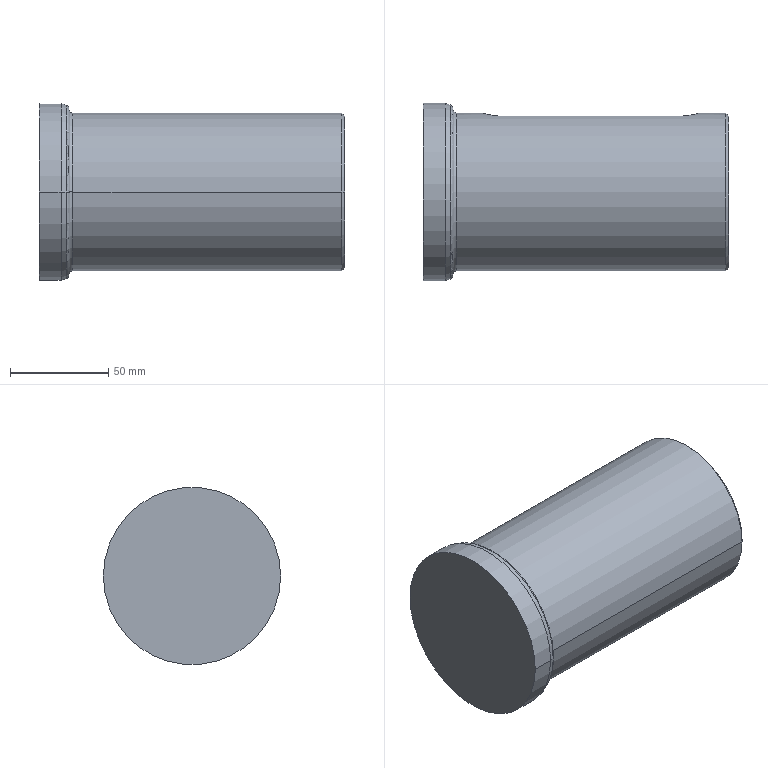Part | STEP file | Input 97 | 1 solid | 31 faces | box 155 x 90 x 90 mm | volume 763007 mm3 | cylinder 11 | cone 8 | torus 6 | plane 6 | commonest cylinder face diameters 22 x3 17.5 x2 21 x2 80 x2 90 x2